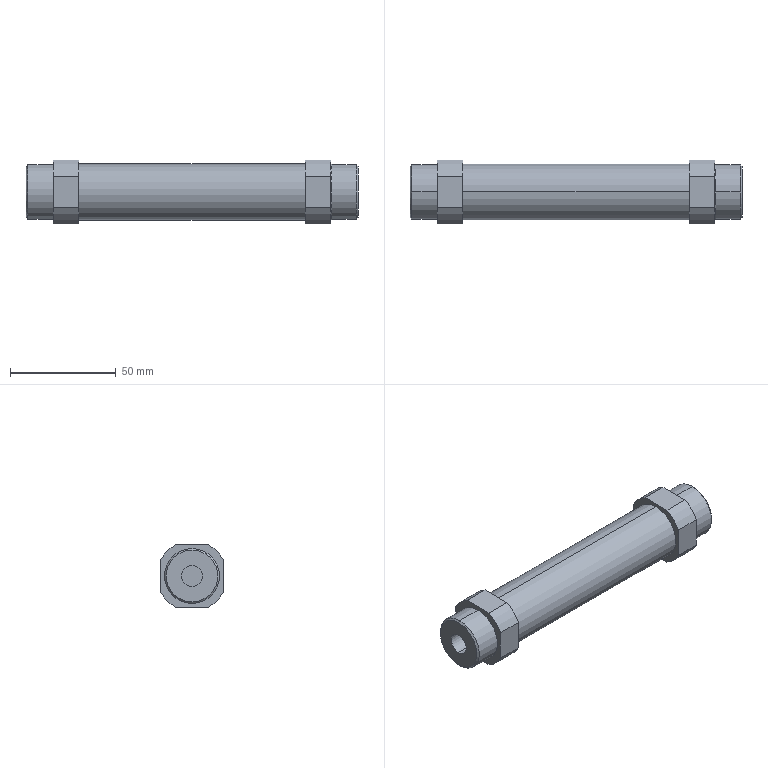Part | SolidWorks | features BaseBody 1 | 1 solid | 52 faces | box 157 x 30 x 30 mm | volume 51247 mm3 | cylinder 22 | plane 16 | cone 12 | spline 2 | commonest cylinder face diameters 33.4 x8 4.134 x4 26 x4 10 x2 25 x2 26.6 x2